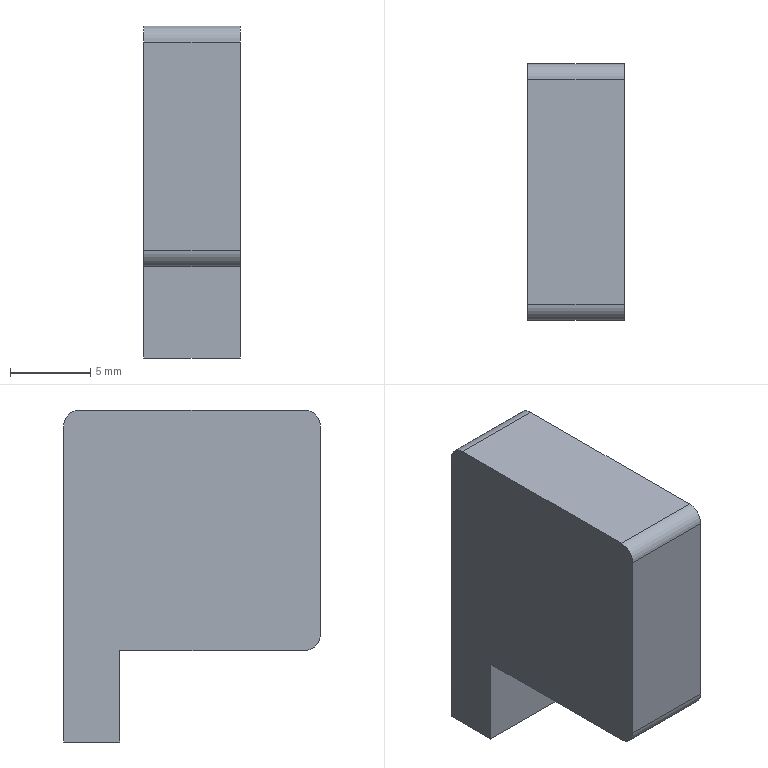Part | SolidWorks | features Fillet 1, FlatPattern 1, SMBaseFlange 1, SheetMetal 1 | 1 solid | 11 faces | box 6 x 16 x 20.7 mm | volume 1556 mm3 | plane 8 | cylinder 3 | commonest cylinder face diameters 2 x3
STEP:
#1=CARTESIAN_POINT('',(0.,0.,-1.));
#2=VERTEX_POINT('',#1);
#3=CARTESIAN_POINT('',(0.,0.,-14.));
#4=VERTEX_POINT('',#3);
#5=CARTESIAN_POINT('',(0.,0.,-15.));
#6=DIRECTION('',(0.,0.,-1.));
#7=VECTOR('',#6,1000.);
#8=LINE('',#5,#7);
#9=EDGE_CURVE('',#2,#4,#8,.T.);
#10=ORIENTED_EDGE('',*,*,#9,.T.);
#11=CARTESIAN_POINT('',(6.,0.,-14.));
#12=VERTEX_POINT('',#11);
#13=CARTESIAN_POINT('',(6.,0.,-14.));
#14=DIRECTION('',(1.,0.,0.));
#15=VECTOR('',#14,1000.);
#16=LINE('',#13,#15);
#17=EDGE_CURVE('',#4,#12,#16,.T.);
#18=ORIENTED_EDGE('',*,*,#17,.T.);
#19=CARTESIAN_POINT('',(6.,0.,-1.));
#20=VERTEX_POINT('',#19);
#21=CARTESIAN_POINT('',(6.,0.,-15.));
#22=DIRECTION('',(0.,0.,-1.));
#23=VECTOR('',#22,1000.);
#24=LINE('',#21,#23);
#25=EDGE_CURVE('',#20,#12,#24,.T.);
#26=ORIENTED_EDGE('',*,*,#25,.F.);
#27=CARTESIAN_POINT('',(6.,0.,-1.));
#28=DIRECTION('',(-1.,0.,0.));
#29=VECTOR('',#28,1000.);
#30=LINE('',#27,#29);
#31=EDGE_CURVE('',#20,#2,#30,.T.);
#32=ORIENTED_EDGE('',*,*,#31,.T.);
#33=EDGE_LOOP('',(#10,#18,#26,#32));
#34=FACE_OUTER_BOUND('',#33,.T.);
#35=CARTESIAN_POINT('',(6.,0.,-15.));
#36=DIRECTION('',(0.,1.,0.));
#37=DIRECTION('',(0.,0.,1.));
#38=AXIS2_PLACEMENT_3D('',#35,#36,#37);
#39=PLANE('',#38);
#40=ADVANCED_FACE('',(#34),#39,.F.);
#41=CARTESIAN_POINT('',(6.,1.,-15.));
#42=VERTEX_POINT('',#41);
#43=CARTESIAN_POINT('',(6.,12.5,-15.));
#44=VERTEX_POINT('',#43);
#45=CARTESIAN_POINT('',(6.,12.5,-15.));
#46=DIRECTION('',(0.,1.,0.));
#47=VECTOR('',#46,1000.);
#48=LINE('',#45,#47);
#49=EDGE_CURVE('',#42,#44,#48,.T.);
#50=ORIENTED_EDGE('',*,*,#49,.F.);
#51=CARTESIAN_POINT('',(0.,1.,-15.));
#52=VERTEX_POINT('',#51);
#53=CARTESIAN_POINT('',(6.,1.,-15.));
#54=DIRECTION('',(-1.,0.,0.));
#55=VECTOR('',#54,1000.);
#56=LINE('',#53,#55);
#57=EDGE_CURVE('',#42,#52,#56,.T.);
#58=ORIENTED_EDGE('',*,*,#57,.T.);
#59=CARTESIAN_POINT('',(0.,12.5,-15.));
#60=VERTEX_POINT('',#59);
#61=CARTESIAN_POINT('',(0.,12.5,-15.));
#62=DIRECTION('',(0.,1.,0.));
#63=VECTOR('',#62,1000.);
#64=LINE('',#61,#63);
#65=EDGE_CURVE('',#52,#60,#64,.T.);
#66=ORIENTED_EDGE('',*,*,#65,.T.);
#67=CARTESIAN_POINT('',(6.,12.5,-15.));
#68=DIRECTION('',(-1.,0.,0.));
#69=VECTOR('',#68,1000.);
#70=LINE('',#67,#69);
#71=EDGE_CURVE('',#44,#60,#70,.T.);
#72=ORIENTED_EDGE('',*,*,#71,.F.);
#73=EDGE_LOOP('',(#50,#58,#66,#72));
#74=FACE_OUTER_BOUND('',#73,.T.);
#75=CARTESIAN_POINT('',(6.,12.5,-15.));
#76=DIRECTION('',(0.,0.,1.));
#77=DIRECTION('',(1.,0.,0.));
#78=AXIS2_PLACEMENT_3D('',#75,#76,#77);
#79=PLANE('',#78);
#80=ADVANCED_FACE('',(#74),#79,.F.);
#81=CARTESIAN_POINT('',(0.,12.5,-20.7));
#82=VERTEX_POINT('',#81);
#83=CARTESIAN_POINT('',(0.,12.5,-20.7));
#84=DIRECTION('',(0.,0.,-1.));
#85=VECTOR('',#84,1000.);
#86=LINE('',#83,#85);
#87=EDGE_CURVE('',#60,#82,#86,.T.);
#88=ORIENTED_EDGE('',*,*,#87,.T.);
#89=CARTESIAN_POINT('',(6.,12.5,-20.7));
#90=VERTEX_POINT('',#89);
#91=CARTESIAN_POINT('',(6.,12.5,-20.7));
#92=DIRECTION('',(-1.,0.,0.));
#93=VECTOR('',#92,1000.);
#94=LINE('',#91,#93);
#95=EDGE_CURVE('',#90,#82,#94,.T.);
#96=ORIENTED_EDGE('',*,*,#95,.F.);
#97=CARTESIAN_POINT('',(6.,12.5,-20.7));
#98=DIRECTION('',(0.,0.,-1.));
#99=VECTOR('',#98,1000.);
#100=LINE('',#97,#99);
#101=EDGE_CURVE('',#44,#90,#100,.T.);
#102=ORIENTED_EDGE('',*,*,#101,.F.);
#103=ORIENTED_EDGE('',*,*,#71,.T.);
#104=EDGE_LOOP('',(#88,#96,#102,#103));
#105=FACE_OUTER_BOUND('',#104,.T.);
#106=CARTESIAN_POINT('',(6.,12.5,-20.7));
#107=DIRECTION('',(0.,1.,0.));
#108=DIRECTION('',(0.,0.,1.));
#109=AXIS2_PLACEMENT_3D('',#106,#107,#108);
#110=PLANE('',#109);
#111=ADVANCED_FACE('',(#105),#110,.F.);
#112=CARTESIAN_POINT('',(0.,16.,-20.7));
#113=VERTEX_POINT('',#112);
#114=CARTESIAN_POINT('',(0.,16.,-20.7));
#115=DIRECTION('',(0.,1.,0.));
#116=VECTOR('',#115,1000.);
#117=LINE('',#114,#116);
#118=EDGE_CURVE('',#82,#113,#117,.T.);
#119=ORIENTED_EDGE('',*,*,#118,.T.);
#120=CARTESIAN_POINT('',(6.,16.,-20.7));
#121=VERTEX_POINT('',#120);
#122=CARTESIAN_POINT('',(6.,16.,-20.7));
#123=DIRECTION('',(-1.,0.,0.));
#124=VECTOR('',#123,1000.);
#125=LINE('',#122,#124);
#126=EDGE_CURVE('',#121,#113,#125,.T.);
#127=ORIENTED_EDGE('',*,*,#126,.F.);
#128=CARTESIAN_POINT('',(6.,16.,-20.7));
#129=DIRECTION('',(0.,1.,0.));
#130=VECTOR('',#129,1000.);
#131=LINE('',#128,#130);
#132=EDGE_CURVE('',#90,#121,#131,.T.);
#133=ORIENTED_EDGE('',*,*,#132,.F.);
#134=ORIENTED_EDGE('',*,*,#95,.T.);
#135=EDGE_LOOP('',(#119,#127,#133,#134));
#136=FACE_OUTER_BOUND('',#135,.T.);
#137=CARTESIAN_POINT('',(6.,16.,-20.7));
#138=DIRECTION('',(0.,0.,1.));
#139=DIRECTION('',(1.,0.,0.));
#140=AXIS2_PLACEMENT_3D('',#137,#138,#139);
#141=PLANE('',#140);
#142=ADVANCED_FACE('',(#136),#141,.F.);
#143=CARTESIAN_POINT('',(0.,16.,-1.));
#144=VERTEX_POINT('',#143);
#145=CARTESIAN_POINT('',(0.,16.,0.));
#146=DIRECTION('',(0.,0.,1.));
#147=VECTOR('',#146,1000.);
#148=LINE('',#145,#147);
#149=EDGE_CURVE('',#113,#144,#148,.T.);
#150=ORIENTED_EDGE('',*,*,#149,.T.);
#151=CARTESIAN_POINT('',(6.,16.,-1.));
#152=VERTEX_POINT('',#151);
#153=CARTESIAN_POINT('',(6.,16.,-1.));
#154=DIRECTION('',(1.,0.,0.));
#155=VECTOR('',#154,1000.);
#156=LINE('',#153,#155);
#157=EDGE_CURVE('',#144,#152,#156,.T.);
#158=ORIENTED_EDGE('',*,*,#157,.T.);
#159=CARTESIAN_POINT('',(6.,16.,0.));
#160=DIRECTION('',(0.,0.,1.));
#161=VECTOR('',#160,1000.);
#162=LINE('',#159,#161);
#163=EDGE_CURVE('',#121,#152,#162,.T.);
#164=ORIENTED_EDGE('',*,*,#163,.F.);
#165=ORIENTED_EDGE('',*,*,#126,.T.);
#166=EDGE_LOOP('',(#150,#158,#164,#165));
#167=FACE_OUTER_BOUND('',#166,.T.);
#168=CARTESIAN_POINT('',(6.,16.,0.));
#169=DIRECTION('',(0.,-1.,0.));
#170=DIRECTION('',(0.,0.,-1.));
#171=AXIS2_PLACEMENT_3D('',#168,#169,#170);
#172=PLANE('',#171);
#173=ADVANCED_FACE('',(#167),#172,.F.);
#174=CARTESIAN_POINT('',(0.,15.,0.));
#175=VERTEX_POINT('',#174);
#176=CARTESIAN_POINT('',(0.,1.,0.));
#177=VERTEX_POINT('',#176);
#178=CARTESIAN_POINT('',(0.,0.,0.));
#179=DIRECTION('',(0.,-1.,0.));
#180=VECTOR('',#179,1000.);
#181=LINE('',#178,#180);
#182=EDGE_CURVE('',#175,#177,#181,.T.);
#183=ORIENTED_EDGE('',*,*,#182,.T.);
#184=CARTESIAN_POINT('',(6.,1.,0.));
#185=VERTEX_POINT('',#184);
#186=CARTESIAN_POINT('',(6.,1.,0.));
#187=DIRECTION('',(1.,0.,0.));
#188=VECTOR('',#187,1000.);
#189=LINE('',#186,#188);
#190=EDGE_CURVE('',#177,#185,#189,.T.);
#191=ORIENTED_EDGE('',*,*,#190,.T.);
#192=CARTESIAN_POINT('',(6.,15.,0.));
#193=VERTEX_POINT('',#192);
#194=CARTESIAN_POINT('',(6.,0.,0.));
#195=DIRECTION('',(0.,-1.,0.));
#196=VECTOR('',#195,1000.);
#197=LINE('',#194,#196);
#198=EDGE_CURVE('',#193,#185,#197,.T.);
#199=ORIENTED_EDGE('',*,*,#198,.F.);
#200=CARTESIAN_POINT('',(6.,15.,0.));
#201=DIRECTION('',(-1.,0.,0.));
#202=VECTOR('',#201,1000.);
#203=LINE('',#200,#202);
#204=EDGE_CURVE('',#193,#175,#203,.T.);
#205=ORIENTED_EDGE('',*,*,#204,.T.);
#206=EDGE_LOOP('',(#183,#191,#199,#205));
#207=FACE_OUTER_BOUND('',#206,.T.);
#208=CARTESIAN_POINT('',(6.,0.,0.));
#209=DIRECTION('',(0.,0.,-1.));
#210=DIRECTION('',(-1.,0.,0.));
#211=AXIS2_PLACEMENT_3D('',#208,#209,#210);
#212=PLANE('',#211);
#213=ADVANCED_FACE('',(#207),#212,.F.);
#214=ORIENTED_EDGE('',*,*,#25,.T.);
#215=CARTESIAN_POINT('',(6.,1.,-14.));
#216=DIRECTION('',(1.,0.,0.));
#217=DIRECTION('',(0.,0.,1.));
#218=AXIS2_PLACEMENT_3D('',#215,#216,#217);
#219=CIRCLE('',#218,1.);
#220=EDGE_CURVE('',#12,#42,#219,.T.);
#221=ORIENTED_EDGE('',*,*,#220,.T.);
#222=ORIENTED_EDGE('',*,*,#49,.T.);
#223=ORIENTED_EDGE('',*,*,#101,.T.);
#224=ORIENTED_EDGE('',*,*,#132,.T.);
#225=ORIENTED_EDGE('',*,*,#163,.T.);
#226=CARTESIAN_POINT('',(6.,15.,-1.));
#227=DIRECTION('',(1.,0.,0.));
#228=DIRECTION('',(0.,0.,1.));
#229=AXIS2_PLACEMENT_3D('',#226,#227,#228);
#230=CIRCLE('',#229,1.);
#231=EDGE_CURVE('',#152,#193,#230,.T.);
#232=ORIENTED_EDGE('',*,*,#231,.T.);
#233=ORIENTED_EDGE('',*,*,#198,.T.);
#234=CARTESIAN_POINT('',(6.,1.,-1.));
#235=DIRECTION('',(1.,0.,0.));
#236=DIRECTION('',(0.,0.,1.));
#237=AXIS2_PLACEMENT_3D('',#234,#235,#236);
#238=CIRCLE('',#237,1.);
#239=EDGE_CURVE('',#185,#20,#238,.T.);
#240=ORIENTED_EDGE('',*,*,#239,.T.);
#241=EDGE_LOOP('',(#214,#221,#222,#223,#224,#225,#232,#233,#240));
#242=FACE_OUTER_BOUND('',#241,.T.);
#243=CARTESIAN_POINT('',(6.,0.,0.));
#244=DIRECTION('',(-1.,0.,0.));
#245=DIRECTION('',(0.,0.,1.));
#246=AXIS2_PLACEMENT_3D('',#243,#244,#245);
#247=PLANE('',#246);
#248=ADVANCED_FACE('',(#242),#247,.F.);
#249=ORIENTED_EDGE('',*,*,#65,.F.);
#250=CARTESIAN_POINT('',(0.,1.,-14.));
#251=DIRECTION('',(-1.,0.,0.));
#252=DIRECTION('',(0.,0.,1.));
#253=AXIS2_PLACEMENT_3D('',#250,#251,#252);
#254=CIRCLE('',#253,1.);
#255=EDGE_CURVE('',#52,#4,#254,.T.);
#256=ORIENTED_EDGE('',*,*,#255,.T.);
#257=ORIENTED_EDGE('',*,*,#9,.F.);
#258=CARTESIAN_POINT('',(0.,1.,-1.));
#259=DIRECTION('',(-1.,0.,0.));
#260=DIRECTION('',(0.,0.,1.));
#261=AXIS2_PLACEMENT_3D('',#258,#259,#260);
#262=CIRCLE('',#261,1.);
#263=EDGE_CURVE('',#2,#177,#262,.T.);
#264=ORIENTED_EDGE('',*,*,#263,.T.);
#265=ORIENTED_EDGE('',*,*,#182,.F.);
#266=CARTESIAN_POINT('',(0.,15.,-1.));
#267=DIRECTION('',(-1.,0.,0.));
#268=DIRECTION('',(0.,0.,1.));
#269=AXIS2_PLACEMENT_3D('',#266,#267,#268);
#270=CIRCLE('',#269,1.);
#271=EDGE_CURVE('',#175,#144,#270,.T.);
#272=ORIENTED_EDGE('',*,*,#271,.T.);
#273=ORIENTED_EDGE('',*,*,#149,.F.);
#274=ORIENTED_EDGE('',*,*,#118,.F.);
#275=ORIENTED_EDGE('',*,*,#87,.F.);
#276=EDGE_LOOP('',(#249,#256,#257,#264,#265,#272,#273,#274,#275));
#277=FACE_OUTER_BOUND('',#276,.T.);
#278=CARTESIAN_POINT('',(0.,0.,0.));
#279=DIRECTION('',(-1.,0.,0.));
#280=DIRECTION('',(0.,0.,1.));
#281=AXIS2_PLACEMENT_3D('',#278,#279,#280);
#282=PLANE('',#281);
#283=ADVANCED_FACE('',(#277),#282,.T.);
#284=ORIENTED_EDGE('',*,*,#220,.F.);
#285=ORIENTED_EDGE('',*,*,#17,.F.);
#286=ORIENTED_EDGE('',*,*,#255,.F.);
#287=ORIENTED_EDGE('',*,*,#57,.F.);
#288=EDGE_LOOP('',(#284,#285,#286,#287));
#289=FACE_OUTER_BOUND('',#288,.T.);
#290=CARTESIAN_POINT('',(6.,1.,-14.));
#291=DIRECTION('',(-1.,0.,0.));
#292=DIRECTION('',(0.,0.,1.));
#293=AXIS2_PLACEMENT_3D('',#290,#291,#292);
#294=CYLINDRICAL_SURFACE('',#293,1.);
#295=ADVANCED_FACE('',(#289),#294,.T.);
#296=ORIENTED_EDGE('',*,*,#239,.F.);
#297=ORIENTED_EDGE('',*,*,#190,.F.);
#298=ORIENTED_EDGE('',*,*,#263,.F.);
#299=ORIENTED_EDGE('',*,*,#31,.F.);
#300=EDGE_LOOP('',(#296,#297,#298,#299));
#301=FACE_OUTER_BOUND('',#300,.T.);
#302=CARTESIAN_POINT('',(6.,1.,-1.));
#303=DIRECTION('',(-1.,0.,0.));
#304=DIRECTION('',(0.,0.,1.));
#305=AXIS2_PLACEMENT_3D('',#302,#303,#304);
#306=CYLINDRICAL_SURFACE('',#305,1.);
#307=ADVANCED_FACE('',(#301),#306,.T.);
#308=ORIENTED_EDGE('',*,*,#231,.F.);
#309=ORIENTED_EDGE('',*,*,#157,.F.);
#310=ORIENTED_EDGE('',*,*,#271,.F.);
#311=ORIENTED_EDGE('',*,*,#204,.F.);
#312=EDGE_LOOP('',(#308,#309,#310,#311));
#313=FACE_OUTER_BOUND('',#312,.T.);
#314=CARTESIAN_POINT('',(6.,15.,-1.));
#315=DIRECTION('',(-1.,0.,0.));
#316=DIRECTION('',(0.,0.,1.));
#317=AXIS2_PLACEMENT_3D('',#314,#315,#316);
#318=CYLINDRICAL_SURFACE('',#317,1.);
#319=ADVANCED_FACE('',(#313),#318,.T.);
#320=CLOSED_SHELL('',(#40,#80,#111,#142,#173,#213,#248,#283,#295,#307,#319));
#321=MANIFOLD_SOLID_BREP('',#320);
#322=CARTESIAN_POINT('',(0.,0.,0.));
#323=DIRECTION('',(0.,0.,1.));
#324=DIRECTION('',(1.,0.,0.));
#325=AXIS2_PLACEMENT_3D('',#322,#323,#324);
#326=(LENGTH_UNIT()NAMED_UNIT(*)SI_UNIT(.MILLI.,.METRE.));
#327=UNCERTAINTY_MEASURE_WITH_UNIT(LENGTH_MEASURE(0.00001),#326,'','');
#328=(NAMED_UNIT(*)PLANE_ANGLE_UNIT()SI_UNIT($,.RADIAN.));
#329=(NAMED_UNIT(*)SI_UNIT($,.STERADIAN.)SOLID_ANGLE_UNIT());
#330=(GEOMETRIC_REPRESENTATION_CONTEXT(3)GLOBAL_UNCERTAINTY_ASSIGNED_CONTEXT((#327))GLOBAL_UNIT_ASSIGNED_CONTEXT((#326,#328,#329))REPRESENTATION_CONTEXT('',''));
#331=ADVANCED_BREP_SHAPE_REPRESENTATION('',(#321,#325),#330);